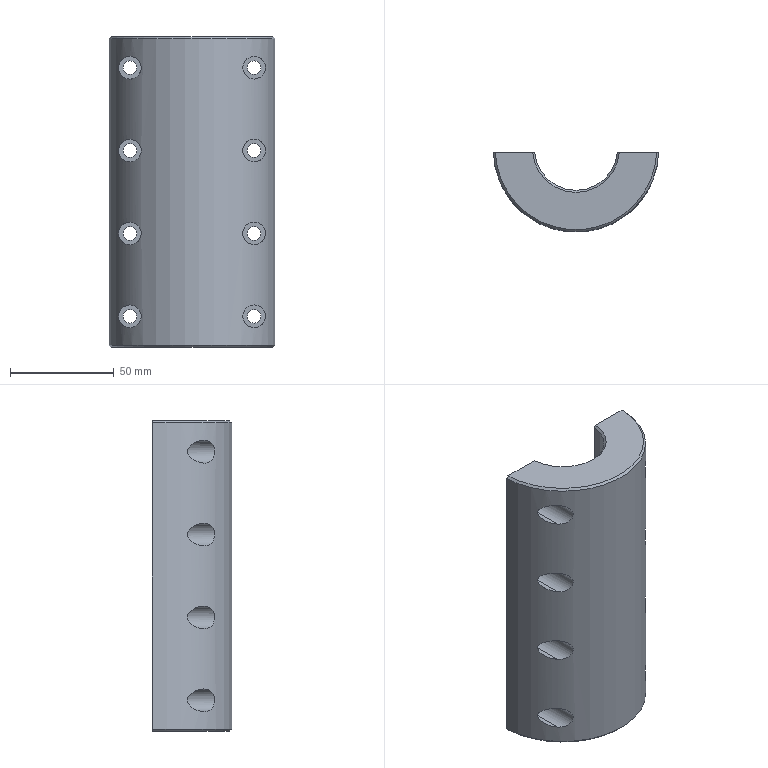Part | SolidWorks | features ICE 2, Chamfer 1, Extrusion 1, HoleWzd 1, LPattern 1 | 1 solid | 50 faces | box 79.944 x 38.5 x 150 mm | volume 259221 mm3 | cylinder 34 | plane 12 | cone 4 | commonest cylinder face diameters 6.6 x16 11 x16 40 x1 80 x1